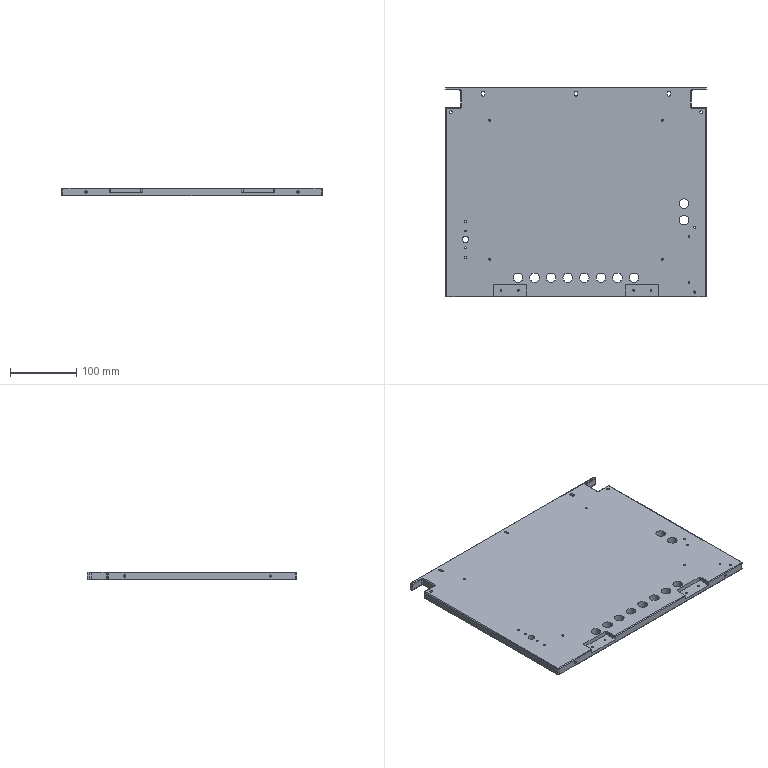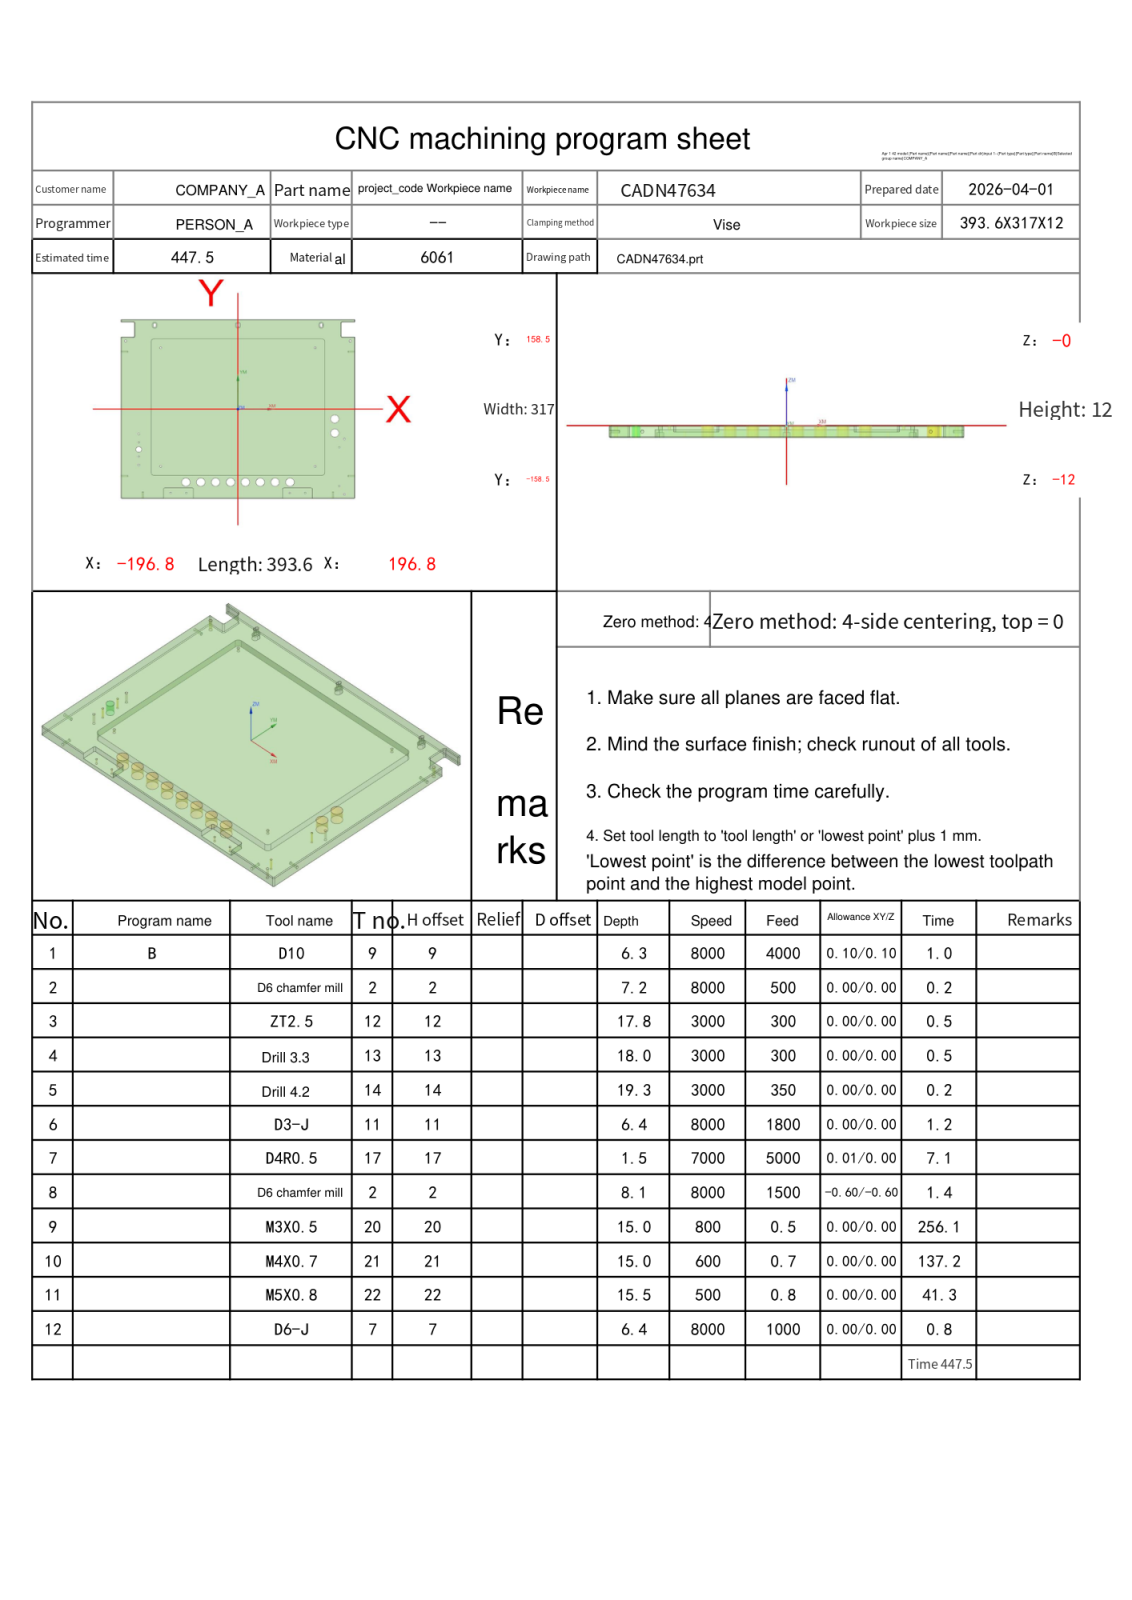NC program | NX | posted by the shop | part box 393.6 x 317 x 12 mm
Lines 5063 to 6733 of 6733:
N7 T17 M06
(D4R0.5  D=4. R=0.5 H=17 ce=0.01 di=0.00)
G00 G90 G54 X-120.803 Y-159.316 M03 S7000
G43 H17 Z10.01
M08
Z.488
G01 Z-.012 F5000.
X-123.9 Y-159.089
G03 X-124.138 Y-159.081 I-.238 J-3.254
X-125. Y-159.197 I0.0 J-3.263
G01 X-194.8
G02 X-197.497 Y-156.5 I0.0 J2.697
G01 Y126.5
G02 X-195.8 Y128.196 I1.697 J0.0
G01 X-175.9
G03 X-174.597 Y129.5 I0.0 J1.303
G01 Y152.
G03 X-175.9 Y153.304 I-1.303 J0.0
G01 X-195.8
G02 X-197.497 Y155.001 I0.0 J1.697
G01 Y157.5
G02 X-195.8 Y159.197 I1.697 J0.0
G01 X195.8
G02 X197.497 Y157.5 I0.0 J-1.697
G01 Y155.001
G02 X195.8 Y153.304 I-1.697 J0.0
G01 X175.9
G03 X174.597 Y152. I0.0 J-1.303
G01 Y129.5
G03 X175.9 Y128.196 I1.303 J0.0
G01 X195.8
G02 X197.497 Y126.5 I0.0 J-1.697
G01 Y-156.5
G02 X194.8 Y-159.197 I-2.697 J0.0
G01 X125.
X124.799 Y-159.126
X123.899 Y-159.084
Y-159.152 Z-.018
X123.9 Z-.025
X125. Y-159.284
X194.8
G03 X197.584 Y-156.5 I0.0 J2.784
G01 Y126.5
G03 X195.8 Y128.284 I-1.784 J0.0
G01 X175.9
G02 X174.685 Y129.5 I0.0 J1.216
G01 Y152.
G02 X175.9 Y153.216 I1.216 J0.0
G01 X195.8
G03 X197.584 Y155.001 I0.0 J1.784
G01 Y157.5
G03 X195.8 Y159.284 I-1.784 J0.0
G01 X-195.8
G03 X-197.584 Y157.5 I0.0 J-1.784
G01 Y155.001
G03 X-195.8 Y153.216 I1.784 J0.0
G01 X-175.9
G02 X-174.685 Y152. I0.0 J-1.216
G01 Y129.5
G02 X-175.9 Y128.284 I-1.216 J0.0
G01 X-195.8
G03 X-197.584 Y126.5 I0.0 J-1.784
G01 Y-156.5
G03 X-194.8 Y-159.284 I2.784 J0.0
G01 X-125.
G02 X-124.067 Y-159.161 I.932 J-3.463
G01 X-123.9 Y-159.165
Y-159.243 Z-.034
Y-159.259 Z-.042
X-124.07 Y-159.255
G03 X-125. Y-159.363 I0.0 J-4.044
G01 X-194.8
G02 X-197.663 Y-156.5 I0.0 J2.863
G01 Y126.5
G02 X-195.8 Y128.363 I1.863 J0.0
G01 X-175.9
G03 X-174.764 Y129.5 I0.0 J1.137
G01 Y152.
G03 X-175.9 Y153.137 I-1.137 J0.0
G01 X-195.8
G02 X-197.663 Y155.001 I0.0 J1.863
G01 Y157.5
G02 X-195.8 Y159.363 I1.863 J0.0
G01 X195.8
G02 X197.663 Y157.5 I0.0 J-1.863
G01 Y155.001
G02 X195.8 Y153.137 I-1.863 J0.0
G01 X175.9
G03 X174.764 Y152. I0.0 J-1.137
G01 Y129.5
G03 X175.9 Y128.363 I1.137 J0.0
G01 X195.8
G02 X197.663 Y126.5 I0.0 J-1.863
G01 Y-156.5
G02 X194.8 Y-159.363 I-2.863 J0.0
G01 X125.
X123.9 Y-159.238
Y-159.293 Z-.053
Y-159.329 Z-.063
X123.949 Y-159.333
X125. Y-159.44
X194.8
G03 X197.74 Y-156.5 I0.0 J2.94
G01 Y126.5
G03 X195.8 Y128.44 I-1.94 J0.0
G01 X175.9
G02 X174.84 Y129.5 I0.0 J1.06
G01 Y152.
G02 X175.9 Y153.06 I1.06 J0.0
G01 X195.8 Y153.061
G03 X197.74 Y155.001 I0.0 J1.94
G01 Y157.5
G03 X195.8 Y159.44 I-1.94 J0.0
G01 X-195.8
G03 X-197.74 Y157.5 I0.0 J-1.94
G01 Y155.001
G03 X-195.8 Y153.061 I1.94 J0.0
G01 X-175.9 Y153.06
G02 X-174.84 Y152. I0.0 J-1.06
G01 Y129.5
G02 X-175.9 Y128.44 I-1.06 J0.0
G01 X-195.8
G03 X-197.74 Y126.5 I0.0 J-1.94
G01 Y-156.5
G03 X-194.8 Y-159.44 I2.94 J0.0
G01 X-125.
G02 X-124.019 Y-159.344 I.981 J-4.998
G01 X-123.9 Y-159.346
X-123.899 Y-159.394 Z-.076
Y-159.426 Z-.089
G03 X-124.115 Y-159.42 I-.216 J-4.053
X-125. Y-159.518 I0.0 J-4.059
G01 X-194.8
G02 X-197.818 Y-156.5 I0.0 J3.018
G01 Y126.5
G02 X-195.8 Y128.518 I2.018 J0.0
G01 X-175.9
G03 X-174.918 Y129.5 I0.0 J.982
G01 Y152.
G03 X-175.9 Y152.982 I-.982 J0.0
G01 X-195.8 Y152.983
G02 X-197.818 Y155.001 I0.0 J2.018
G01 Y157.5
G02 X-195.8 Y159.518 I2.018 J0.0
G01 X195.8
G02 X197.818 Y157.5 I0.0 J-2.018
G01 Y155.001
G02 X195.8 Y152.983 I-2.018 J0.0
G01 X175.9 Y152.982
G03 X174.918 Y152. I0.0 J-.982
G01 Y129.5
G03 X175.9 Y128.518 I.982 J0.0
G01 X195.8
G02 X197.818 Y126.5 I0.0 J-2.018
G01 Y-156.5
G02 X194.8 Y-159.518 I-3.018 J0.0
G01 X125.
G03 X123.898 Y-159.403 I-1.187 J-6.06
G01 Y-159.446 Z-.104
Y-159.483 Z-.12
G02 X125. Y-159.597 I-.142 J-6.724
G01 X194.8
G03 X197.897 Y-156.5 I0.0 J3.097
G01 Y126.5
G03 X195.8 Y128.597 I-2.097 J0.0
G01 X175.9
G02 X174.997 Y129.5 I0.0 J.903
G01 Y152.
G02 X175.9 Y152.903 I.903 J0.0
G01 X195.8 Y152.904
G03 X197.897 Y155.001 I0.0 J2.097
G01 Y157.5
G03 X195.8 Y159.597 I-2.097 J0.0
G01 X-195.8
G03 X-197.897 Y157.5 I0.0 J-2.097
G01 Y155.001
G03 X-195.8 Y152.904 I2.097 J0.0
G01 X-175.9 Y152.903
G02 X-174.997 Y152. I0.0 J-.903
G01 Y129.5
G02 X-175.9 Y128.597 I-.903 J0.0
G01 X-195.8
G03 X-197.897 Y126.5 I0.0 J-2.097
G01 Y-156.5
G03 X-194.8 Y-159.597 I3.097 J0.0
G01 X-125.
G02 X-124.051 Y-159.497 I.949 J-4.449
G01 X-123.899 Y-159.5
X-123.9 Y-159.542 Z-.138
Y-159.576 Z-.156
G03 X-125. Y-159.677 I.01 J-6.176
G01 X-194.8
G02 X-197.977 Y-156.5 I0.0 J3.177
G01 Y126.5
G02 X-195.8 Y128.676 I2.177 J0.0
G01 X-175.9
G03 X-175.077 Y129.5 I0.0 J.823
G01 Y152.
G03 X-175.9 Y152.824 I-.823 J0.0
G01 X-195.8
G02 X-197.977 Y155.001 I0.0 J2.177
G01 Y157.5
G02 X-195.8 Y159.677 I2.177 J0.0
G01 X195.8
G02 X197.977 Y157.5 I0.0 J-2.177
G01 Y155.001
G02 X195.8 Y152.824 I-2.177 J0.0
G01 X175.9
G03 X175.077 Y152. I0.0 J-.823
G01 Y129.5
G03 X175.9 Y128.676 I.823 J0.0
G01 X195.8
G02 X197.977 Y126.5 I0.0 J-2.177
G01 Y-156.5
G02 X194.8 Y-159.677 I-3.177 J0.0
G01 X125.
G03 X123.9 Y-159.565 I-1.385 J-8.202
G01 X123.899 Y-159.615 Z-.177
Y-159.657 Z-.198
G02 X125. Y-159.755 I-.262 J-9.172
G01 X194.8
G03 X198.055 Y-156.5 I0.0 J3.255
G01 Y126.5
G03 X195.8 Y128.755 I-2.255 J0.0
G01 X175.9
G02 X175.155 Y129.5 I0.0 J.745
G01 Y152.
G02 X175.9 Y152.745 I.745 J0.0
G01 X195.8 Y152.746
G03 X198.055 Y155.001 I0.0 J2.255
G01 Y157.5
G03 X195.8 Y159.755 I-2.255 J0.0
G01 X-195.8
G03 X-198.055 Y157.5 I0.0 J-2.255
G01 Y155.001
G03 X-195.8 Y152.746 I2.255 J0.0
G01 X-175.9 Y152.745
G02 X-175.155 Y152. I0.0 J-.745
G01 Y129.5
G02 X-175.9 Y128.755 I-.745 J0.0
G01 X-195.8
G03 X-198.055 Y126.5 I0.0 J-2.255
G01 Y-156.5
G03 X-194.8 Y-159.755 I3.255 J0.0
G01 X-125.
G02 X-123.899 Y-159.661 I1.326 J-9.063
G01 Y-159.71 Z-.222
Y-159.753 Z-.247
G03 X-125. Y-159.834 I.089 J-8.636
G01 X-194.8
G02 X-198.134 Y-156.5 I0.0 J3.334
G01 Y126.5
G02 X-195.8 Y128.834 I2.334 J0.0
G01 X-175.9
G03 X-175.235 Y129.5 I0.0 J.666
G01 Y152.
G03 X-175.9 Y152.666 I-.666 J0.0
G01 X-195.8
G02 X-198.134 Y155.001 I0.0 J2.334
G01 Y157.5
G02 X-195.8 Y159.834 I2.334 J0.0
G01 X195.8
G02 X198.134 Y157.5 I0.0 J-2.334
G01 Y155.001
G02 X195.8 Y152.666 I-2.334 J0.0
G01 X175.9
G03 X175.235 Y152. I0.0 J-.666
G01 Y129.5
G03 X175.9 Y128.834 I.666 J0.0
G01 X195.8
G02 X198.134 Y126.5 I0.0 J-2.334
G01 Y-156.5
G02 X194.8 Y-159.834 I-3.334 J0.0
G01 X125.
G03 X123.899 Y-159.752 I-1.11 J-7.483
G01 Y-159.794 Z-.274
X123.9 Y-159.827 Z-.301
G02 X125. Y-159.912 I-.128 J-8.894
G01 X194.8
G03 X198.212 Y-156.5 I0.0 J3.412
G01 Y126.5
G03 X195.8 Y128.912 I-2.412 J0.0
G01 X175.9
G02 X175.312 Y129.5 I0.0 J.588
G01 Y152.
G02 X175.9 Y152.588 I.588 J0.0
G01 X195.8 Y152.589
G03 X198.212 Y155.001 I0.0 J2.412
G01 Y157.5
G03 X195.8 Y159.912 I-2.412 J0.0
G01 X-195.8
G03 X-198.212 Y157.5 I0.0 J-2.412
G01 Y155.001
G03 X-195.8 Y152.589 I2.412 J0.0
G01 X-175.9 Y152.588
G02 X-175.312 Y152. I0.0 J-.588
G01 Y129.5
G02 X-175.9 Y128.912 I-.588 J0.0
G01 X-195.8
G03 X-198.212 Y126.5 I0.0 J-2.412
G01 Y-156.5
G03 X-194.8 Y-159.912 I3.412 J0.0
G01 X-125.
G02 X-123.9 Y-159.827 I1.229 J-8.808
G01 Y-159.872 Z-.331
Y-159.908 Z-.361
G03 X-125. Y-159.986 I.01 J-7.869
G01 X-194.8
G02 X-198.286 Y-156.5 I0.0 J3.486
G01 Y126.5
G02 X-195.8 Y128.986 I2.486 J0.0
G01 X-175.9
G03 X-175.386 Y129.5 I0.0 J.514
G01 Y152.
G03 X-175.9 Y152.514 I-.514 J0.0
G01 X-195.8 Y152.515
G02 X-198.286 Y155.001 I0.0 J2.486
G01 Y157.5
G02 X-195.8 Y159.986 I2.486 J0.0
G01 X195.8
G02 X198.286 Y157.5 I0.0 J-2.486
G01 Y155.001
G02 X195.8 Y152.515 I-2.486 J0.0
G01 X175.9 Y152.514
G03 X175.386 Y152. I0.0 J-.514
G01 Y129.5
G03 X175.9 Y128.986 I.514 J0.0
G01 X195.8
G02 X198.286 Y126.5 I0.0 J-2.486
G01 Y-156.5
G02 X194.8 Y-159.986 I-3.486 J0.0
G01 X125.
G03 X123.9 Y-159.908 I-1.11 J-7.791
G01 X123.899 Y-159.953 Z-.394
Y-159.991 Z-.426
G02 X125. Y-160.058 I-.091 J-10.664
G01 X194.8
G03 X198.358 Y-156.5 I0.0 J3.558
G01 Y126.5
G03 X195.8 Y129.057 I-2.558 J0.0
G01 X175.9
G02 X175.458 Y129.5 I0.0 J.442
G01 Y152.
G02 X175.9 Y152.443 I.442 J0.0
G01 X195.8
G03 X198.358 Y155.001 I0.0 J2.558
G01 Y157.5
G03 X195.8 Y160.058 I-2.558 J0.0
G01 X-195.8
G03 X-198.358 Y157.5 I0.0 J-2.558
G01 Y155.001
G03 X-195.8 Y152.443 I2.558 J0.0
G01 X-175.9
G02 X-175.458 Y152. I0.0 J-.442
G01 Y129.5
G02 X-175.9 Y129.057 I-.442 J0.0
G01 X-195.8
G03 X-198.358 Y126.5 I0.0 J-2.558
G01 Y-156.5
G03 X-194.8 Y-160.058 I3.558 J0.0
G01 X-125.
G02 X-123.899 Y-159.991 I1.192 J-10.596
G01 Y-160.03 Z-.462
Y-160.06 Z-.497
X-123.956
G03 X-125. Y-160.125 I0.0 J-8.34
G01 X-194.8
G02 X-198.425 Y-156.5 I0.0 J3.625
G01 Y126.5
G02 X-195.8 Y129.125 I2.625 J0.0
G01 X-175.9
G03 X-175.525 Y129.5 I0.0 J.375
G01 Y152.
G03 X-175.9 Y152.375 I-.375 J0.0
G01 X-195.8
G02 X-198.425 Y155.001 I0.0 J2.625
G01 Y157.5
G02 X-195.8 Y160.125 I2.625 J0.0
G01 X195.8
G02 X198.425 Y157.5 I0.0 J-2.625
G01 Y155.001
G02 X195.8 Y152.375 I-2.625 J0.0
G01 X175.9
G03 X175.525 Y152. I0.0 J-.375
G01 Y129.5
G03 X175.9 Y129.125 I.375 J0.0
G01 X195.8
G02 X198.425 Y126.5 I0.0 J-2.625
G01 Y-156.5
G02 X194.8 Y-160.125 I-3.625 J0.0
G01 X125.
G03 X123.956 Y-160.06 I-1.044 J-8.275
G01 X123.899
X123.9 Y-160.097 Z-.535
Y-160.122 Z-.572
G02 X125. Y-160.189 I-.149 J-11.663
G01 X194.8
G03 X198.489 Y-156.5 I0.0 J3.689
G01 Y126.5
G03 X195.8 Y129.188 I-2.689 J0.0
G01 X175.9
G02 X175.589 Y129.5 I0.0 J.311
G01 Y152.
G02 X175.9 Y152.312 I.311 J0.0
G01 X195.8
G03 X198.489 Y155.001 I0.0 J2.689
G01 Y157.5
G03 X195.8 Y160.189 I-2.689 J0.0
G01 X-195.8
G03 X-198.489 Y157.5 I0.0 J-2.689
G01 Y155.001
G03 X-195.8 Y152.312 I2.689 J0.0
G01 X-175.9
G02 X-175.589 Y152. I0.0 J-.311
G01 Y129.5
G02 X-175.9 Y129.188 I-.311 J0.0
G01 X-195.8
G03 X-198.489 Y126.5 I0.0 J-2.689
G01 Y-156.5
G03 X-194.8 Y-160.189 I3.689 J0.0
G01 X-125.
G02 X-123.9 Y-160.122 I1.249 J-11.596
G01 Y-160.158 Z-.612
Y-160.186 Z-.651
X-124.003
G03 X-125. Y-160.247 I0.0 J-8.137
G01 X-194.8
G02 X-198.547 Y-156.5 I0.0 J3.747
G01 Y126.5
G02 X-195.8 Y129.247 I2.747 J0.0
G01 X-175.9
G03 X-175.647 Y129.5 I0.0 J.253
G01 Y152.
G03 X-175.9 Y152.253 I-.253 J0.0
G01 X-195.8 Y152.254
G02 X-198.547 Y155.001 I0.0 J2.747
G01 Y157.5
G02 X-195.8 Y160.247 I2.747 J0.0
G01 X195.8
G02 X198.547 Y157.5 I0.0 J-2.747
G01 Y155.001
G02 X195.8 Y152.254 I-2.747 J0.0
G01 X175.9 Y152.253
G03 X175.647 Y152. I0.0 J-.253
G01 Y129.5
G03 X175.9 Y129.247 I.253 J0.0
G01 X195.8
G02 X198.547 Y126.5 I0.0 J-2.747
G01 Y-156.5
G02 X194.8 Y-160.247 I-3.747 J0.0
G01 X125.
G03 X124.003 Y-160.186 I-.997 J-8.075
G01 X123.9
X123.899 Y-160.22 Z-.693
Y-160.246 Z-.735
X123.979
G02 X125. Y-160.3 I0.0 J-9.614
G01 X194.8
G03 X198.6 Y-156.5 I0.0 J3.8
G01 Y126.5
G03 X195.8 Y129.3 I-2.8 J0.0
G01 X175.9
G02 X175.7 Y129.5 I0.0 J.2
G01 Y152.
G02 X175.9 Y152.2 I.2 J0.0
G01 X195.8 Y152.201
G03 X198.6 Y155.001 I0.0 J2.8
G01 Y157.5
G03 X195.8 Y160.3 I-2.8 J0.0
G01 X-195.8
G03 X-198.6 Y157.5 I0.0 J-2.8
G01 Y155.001
G03 X-195.8 Y152.201 I2.8 J0.0
G01 X-175.9 Y152.2
G02 X-175.7 Y152. I0.0 J-.2
G01 Y129.5
G02 X-175.9 Y129.3 I-.2 J0.0
G01 X-195.8
G03 X-198.6 Y126.5 I0.0 J-2.8
G01 Y-156.5
G03 X-194.8 Y-160.3 I3.8 J0.0
G01 X-125.
G02 X-123.977 Y-160.246 I1.023 J-9.576
G01 X-123.899
Y-160.272 Z-.778
X-123.898 Y-160.296 Z-.822
G03 X-125. Y-160.348 I.004 J-11.898
G01 X-194.8
G02 X-198.648 Y-156.5 I0.0 J3.848
G01 Y126.5
G02 X-195.8 Y129.348 I2.848 J0.0
G01 X-175.9
G03 X-175.748 Y129.5 I0.0 J.152
G01 Y152.
G03 X-175.9 Y152.152 I-.152 J0.0
G01 X-195.8 Y152.153
G02 X-198.648 Y155.001 I0.0 J2.848
G01 Y157.5
G02 X-195.8 Y160.348 I2.848 J0.0
G01 X195.8
G02 X198.648 Y157.5 I0.0 J-2.848
G01 Y155.001
G02 X195.8 Y152.153 I-2.848 J0.0
G01 X175.9 Y152.152
G03 X175.748 Y152. I0.0 J-.152
G01 Y129.5
G03 X175.9 Y129.348 I.152 J0.0
G01 X195.8
G02 X198.648 Y126.5 I0.0 J-2.848
G01 Y-156.5
G02 X194.8 Y-160.348 I-3.848 J0.0
G01 X125.
G03 X123.926 Y-160.297 I-1.074 J-11.297
G01 X123.899
Y-160.323 Z-.867
Y-160.342 Z-.912
G02 X124.143 Y-160.338 I.244 J-8.366
X124.516 Y-160.347 I0.0 J-8.369
G03 X125. Y-160.39 I.616 J4.15
G01 X194.8
G03 X198.69 Y-156.5 I0.0 J3.89
G01 Y126.5
G03 X195.8 Y129.39 I-2.89 J0.0
G01 X175.9
X175.84 Y129.396
X175.796 Y129.44
X175.79 Y129.5
Y152.
X175.796 Y152.06
X175.84 Y152.104
X175.9 Y152.11
X195.8 Y152.111
G03 X198.69 Y155.001 I0.0 J2.89
G01 Y157.5
G03 X195.8 Y160.39 I-2.89 J0.0
G01 X-195.8
G03 X-198.69 Y157.5 I0.0 J-2.89
G01 Y155.001
G03 X-195.8 Y152.111 I2.89 J0.0
G01 X-175.9 Y152.11
X-175.84 Y152.104
X-175.796 Y152.06
X-175.79 Y152.
Y129.5
X-175.796 Y129.44
X-175.84 Y129.396
X-175.9 Y129.39
X-195.8
G03 X-198.69 Y126.5 I0.0 J-2.89
G01 Y-156.5
G03 X-194.8 Y-160.39 I3.89 J0.0
G01 X-125.
G03 X-124.516 Y-160.349 I-.173 J4.958
G01 X-123.899 Y-160.336
Y-160.36 Z-.959
Y-160.374 Z-1.005
X-123.91
G03 X-125. Y-160.426 I0.0 J-11.544
G01 X-194.8
G02 X-198.726 Y-156.5 I0.0 J3.926
G01 Y126.5
G02 X-195.8 Y129.426 I2.926 J0.0
G01 X-175.9
X-175.858 Y129.427
X-175.827 Y129.458
X-175.826 Y129.5
Y152.
X-175.827 Y152.042
X-175.858 Y152.073
X-175.9 Y152.074
X-195.8 Y152.075
G02 X-198.726 Y155.001 I0.0 J2.926
G01 Y157.5
G02 X-195.8 Y160.426 I2.926 J0.0
G01 X195.8
G02 X198.726 Y157.5 I0.0 J-2.926
G01 Y155.001
G02 X195.8 Y152.075 I-2.926 J0.0
G01 X175.9 Y152.074
X175.858 Y152.073
X175.827 Y152.042
X175.826 Y152.
Y129.5
X175.827 Y129.458
X175.858 Y129.427
X175.9 Y129.426
X195.8
G02 X198.726 Y126.5 I0.0 J-2.926
G01 Y-156.5
G02 X194.8 Y-160.426 I-3.926 J0.0
G01 X125.
X124.666 Y-160.397
G03 X124.199 Y-160.376 I-.466 J-5.296
X123.899 Y-160.385 I0.0 J-5.317
G01 X123.9 Y-160.412 Z-1.053
Y-160.422 Z-1.1
G02 X124.216 Y-160.417 I.317 J-9.912
X124.516 Y-160.421 I0.0 J-9.917
G03 X125. Y-160.456 I.618 J5.232
G01 X194.8
G03 X198.756 Y-156.5 I0.0 J3.956
G01 Y126.5
G03 X195.8 Y129.456 I-2.956 J0.0
G01 X175.9
X175.873 Y129.453
X175.853 Y129.473
X175.856 Y129.5
Y152.
X175.853 Y152.027
X175.873 Y152.047
X175.9 Y152.044
X195.8 Y152.045
G03 X198.756 Y155.001 I0.0 J2.956
G01 Y157.5
G03 X195.8 Y160.456 I-2.956 J0.0
G01 X-195.8
G03 X-198.756 Y157.5 I0.0 J-2.956
G01 Y155.001
G03 X-195.8 Y152.045 I2.956 J0.0
G01 X-175.9 Y152.044
X-175.873 Y152.047
X-175.853 Y152.027
X-175.856 Y152.
Y129.5
X-175.853 Y129.473
X-175.873 Y129.453
X-175.9 Y129.456
X-195.8
G03 X-198.756 Y126.5 I0.0 J-2.956
G01 Y-156.5
G03 X-194.8 Y-160.456 I3.956 J0.0
G01 X-125.
G02 X-123.9 Y-160.413 I1.382 J-21.397
G01 Y-160.436 Z-1.149
Y-160.45 Z-1.198
X-124.799 Y-160.471
X-125. Y-160.479
X-194.8
G02 X-198.779 Y-156.5 I0.0 J3.979
G01 Y126.5
G02 X-195.8 Y129.479 I2.979 J0.0
G01 X-175.9
X-175.878 Y129.478
X-175.879 Y129.5
Y152.
X-175.878 Y152.022
X-175.9 Y152.021
X-195.8 Y152.022
G02 X-198.779 Y155.001 I0.0 J2.979
G01 Y157.5
G02 X-195.8 Y160.479 I2.979 J0.0
G01 X195.8
G02 X198.779 Y157.5 I0.0 J-2.979
G01 Y155.001
G02 X195.8 Y152.022 I-2.979 J0.0
G01 X175.9 Y152.021
X175.878 Y152.022
X175.879 Y152.
Y129.5
X175.878 Y129.478
X175.9 Y129.479
X195.8
G02 X198.779 Y126.5 I0.0 J-2.979
G01 Y-156.5
G02 X194.8 Y-160.479 I-3.979 J0.0
G01 X125.
G03 X124.184 Y-160.452 I-.816 J-12.346
X123.901 Y-160.455 I0.0 J-12.373
G01 X123.902 Y-160.469 Z-1.235
Y-160.475 Z-1.273
G02 X124.157 Y-160.473 I.255 J-18.193
X125. Y-160.493 I0.0 J-18.194
G01 X194.8
G03 X198.793 Y-156.5 I0.0 J3.993
G01 Y126.5
G03 X195.8 Y129.493 I-2.993 J0.0
G01 X175.9
X175.892 Y129.492
X175.893 Y129.5
Y152.
X175.892 Y152.008
X175.9 Y152.007
X195.8 Y152.008
G03 X198.793 Y155.001 I0.0 J2.993
G01 Y157.5
G03 X195.8 Y160.493 I-2.993 J0.0
G01 X-195.8
G03 X-198.793 Y157.5 I0.0 J-2.993
G01 Y155.001
G03 X-195.8 Y152.008 I2.993 J0.0
G01 X-175.9 Y152.007
X-175.892 Y152.008
X-175.893 Y152.
Y129.5
X-175.892 Y129.492
X-175.9 Y129.493
X-195.8
G03 X-198.793 Y126.5 I0.0 J-2.993
G01 Y-156.5
G03 X-194.8 Y-160.493 I3.993 J0.0
G01 X-125.
X-124.799 Y-160.484
X-123.902 Y-160.47
X-123.903 Y-160.481 Z-1.311
X-123.904 Y-160.485 Z-1.349
X-123.949 Y-160.488
X-124.799 Y-160.493
X-125. Y-160.502
X-194.8
G02 X-198.802 Y-156.5 I0.0 J4.002
G01 Y126.5
G02 X-195.8 Y129.502 I3.002 J0.0
G01 X-175.902
Y151.998
X-195.8
G02 X-198.802 Y155.001 I0.0 J3.002
G01 Y157.5
G02 X-195.8 Y160.502 I3.002 J0.0
G01 X195.8
G02 X198.802 Y157.5 I0.0 J-3.002
G01 Y155.001
G02 X195.8 Y151.998 I-3.002 J0.0
G01 X175.902
Y129.502
X195.8
G02 X198.802 Y126.5 I0.0 J-3.002
G01 Y-156.5
G02 X194.8 Y-160.502 I-4.002 J0.0
G01 X125.
X124.799 Y-160.493
X123.905 Y-160.487
X123.906 Y-160.495 Z-1.387
X123.907 Y-160.5 Z-1.424
X123.949 Y-160.502
X124.799 Y-160.503
X125. Y-160.508
X194.8
G03 X198.808 Y-156.5 I0.0 J4.008
G01 Y126.5
G03 X195.8 Y129.508 I-3.008 J0.0
G01 X175.908
Y151.992
X195.8 Y151.993
G03 X198.808 Y155.001 I0.0 J3.008
G01 Y157.5
G03 X195.8 Y160.508 I-3.008 J0.0
G01 X-195.8
G03 X-198.808 Y157.5 I0.0 J-3.008
G01 Y155.001
G03 X-195.8 Y151.993 I3.008 J0.0
G01 X-175.908 Y151.992
Y129.508
X-195.8
G03 X-198.808 Y126.5 I0.0 J-3.008
G01 Y-156.5
G03 X-194.8 Y-160.508 I4.008 J0.0
G01 X-125.
X-124.799 Y-160.503
X-123.949 Y-160.501
X-123.906 Y-160.499
X-123.909 Y-160.507 Z-1.5
X-194.81 Y-160.51
G02 X-198.744 Y-157.224 I.011 J4.011
X-198.81 Y-156.5 I3.97 J.724
G01 X-198.807 Y126.638
G02 X-196.194 Y129.484 I3.007 J-.139
X-195.818 Y129.509 I.376 J-2.828
G01 X-195.81
X-175.924 Y129.51
X-175.912 Y129.513
X-175.911 Y129.525
Y151.988
X-175.925 Y151.99
X-177.495
X-195.8 Y151.991
G02 X-198.796 Y154.708 I0.0 J3.01
G01 X-198.806 Y154.862
X-198.809 Y154.991
X-198.81 Y157.5
X-198.806 Y157.646
G02 X-195.969 Y160.505 I3.006 J-.146
G01 X195.8 Y160.51
X196.045 Y160.5
G02 X198.806 Y157.646 I-.245 J-3.
G01 X198.81 Y157.5
X198.809 Y154.991
X198.807 Y154.862
G02 X195.944 Y151.994 I-3.007 J.138
G01 X175.911 Y151.988
X175.91 Y151.958
X175.911 Y129.525
X175.912 Y129.513
X175.924 Y129.51
X195.81 Y129.509
X195.813
G02 X196.194 Y129.484 I0.0 J-2.922
X198.807 Y126.638 I-.394 J-2.984
G01 X198.81 Y-156.505
G02 X198.742 Y-157.234 I-3.98 J0.0
X194.81 Y-160.51 I-3.943 J.735
G01 X123.91 Y-160.507
G00 Z10.01
X79.118 Y-159.445
Z.488
G01 Z-.012
X76.1 Y-159.087
X75. Y-159.197
X-75.
G03 X-75.963 Y-159.08 I-.963 J-3.914
G01 X-76.1 Y-159.082
Y-159.149 Z-.025
X-75. Y-159.284
X75.
X76.1 Y-159.159
Y-159.235 Z-.034
Y-159.249 Z-.042
X75. Y-159.363
X-75.
X-76.1 Y-159.231
Y-159.285 Z-.053
Y-159.322 Z-.063
X-75. Y-159.44
X75.
G02 X76.1 Y-159.339 I1.134 J-6.292
G01 X76.101 Y-159.384 Z-.076
Y-159.417 Z-.089
X76.006 Y-159.416
G03 X75. Y-159.518 I0.0 J-5.045
G01 X-75.
X-76.069 Y-159.389
X-76.1 Y-159.387
Y-159.437 Z-.104
Y-159.466 Z-.12
X-75. Y-159.597
X75.
G02 X76.026 Y-159.494 I1.026 J-5.055
G01 X76.101 Y-159.495
X76.1 Y-159.537 Z-.138
Y-159.573 Z-.156
G03 X75. Y-159.677 I.042 J-6.341
G01 X-75.
G03 X-76.1 Y-159.559 I-1.59 J-9.655
G01 Y-159.613 Z-.177
X-76.101 Y-159.656 Z-.198
G02 X-75. Y-159.755 I-.281 J-9.276
G01 X75.
G02 X76.101 Y-159.661 I1.247 J-8.074
G01 Y-159.709 Z-.222
Y-159.753 Z-.247
G03 X75. Y-159.834 I.005 J-7.561
G01 X-75.
G03 X-76.101 Y-159.753 I-1.106 J-7.483
G01 Y-159.794 Z-.274
Y-159.828 Z-.301
G02 X-75. Y-159.912 I-.126 J-8.941
G01 X75.
G02 X76.1 Y-159.828 I1.227 J-8.856
G01 Y-159.872 Z-.331
Y-159.908 Z-.361
G03 X75. Y-159.986 I0.0 J-7.79
G01 X-75.
G03 X-76.099 Y-159.908 I-1.099 J-7.713
G01 X-76.101 Y-159.953 Z-.394
X-76.102 Y-159.992 Z-.426
G02 X-75. Y-160.058 I-.06 J-10.274
G01 X75.
G02 X76.101 Y-159.992 I1.161 J-10.207
G01 Y-160.03 Z-.462
Y-160.06 Z-.497
X76.034
G03 X75. Y-160.125 I0.0 J-8.236
G01 X-75.
G03 X-76.034 Y-160.06 I-1.034 J-8.172
G01 X-76.101
Y-160.097 Z-.535
X-76.1 Y-160.123 Z-.572
G02 X-75. Y-160.189 I-.123 J-11.351
G01 X75.
G02 X76.1 Y-160.123 I1.223 J-11.284
G01 Y-160.158 Z-.612
Y-160.187 Z-.651
X75.983 Y-160.186
G03 X75. Y-160.247 I0.0 J-7.968
G01 X-75.
G03 X-75.982 Y-160.186 I-.982 J-7.905
G01 X-76.1 Y-160.187
X-76.101 Y-160.22 Z-.693
Y-160.247 Z-.735
X-75.997 Y-160.246
G02 X-75. Y-160.3 I0.0 J-9.222
G01 X75.
G02 X75.999 Y-160.246 I.999 J-9.191
G01 X76.101 Y-160.247
X76.102 Y-160.272 Z-.778
Y-160.297 Z-.822
X76.074
G03 X75. Y-160.348 I0.0 J-11.388
G01 X-75.
G03 X-76.054 Y-160.298 I-1.054 J-11.047
G01 X-76.102
X-76.101 Y-160.322 Z-.867
Y-160.338 Z-.912
X-75.503 Y-160.346
G03 X-75. Y-160.39 I.682 J4.912
G01 X75.
G03 X75.503 Y-160.348 I-.22 J5.664
G01 X76.101 Y-160.335
Y-160.359 Z-.959
Y-160.373 Z-1.005
G03 X75. Y-160.426 I.018 J-11.906
G01 X-75.
X-75.503 Y-160.384
X-76.1 Y-160.378
Y-160.404 Z-1.053
Y-160.418 Z-1.1
X-75.503 Y-160.422
G03 X-75. Y-160.456 I.638 J5.776
G01 X75.
G02 X76.1 Y-160.412 I1.457 J-22.555
G01 Y-160.434 Z-1.149
Y-160.449 Z-1.198
X75.22 Y-160.471
X75. Y-160.479
X-75.
G03 X-75.916 Y-160.453 I-.916 J-15.962
G01 X-76.1 Y-160.454
X-76.099 Y-160.461 Z-1.235
Y-160.475 Z-1.273
X-75.22 Y-160.482
X-75. Y-160.493
X75.
X75.22 Y-160.484
X76.099 Y-160.469
Y-160.48 Z-1.311
X76.098 Y-160.485 Z-1.349
X75.22 Y-160.493
X75. Y-160.502
X-75.
X-75.22 Y-160.493
X-76.098 Y-160.487
Y-160.496 Z-1.387
X-76.097 Y-160.5 Z-1.424
X-75. Y-160.508
X75.
X76.097 Y-160.499
X76.096 Y-160.508 Z-1.5
X-76.095
G00 Z10.01
G91 G28 Z0.0
M05
M09
G91 G28 Z0.0
M01
N8 T02 M06
(D6 chamfer mill D=6. R=0. H=02 ce=-0.30 di=0.00)
G00 G90 G54 X-164.146 Y-68.114 M03 S7000
G43 H02 Z20.
M08
Z2.5
G01 X-164.155 Y-68.106 Z2.495 F1500.
X-164.511 Y-67.856 Z2.337
X-164.789 Y-67.696 Z2.22
X-165.183 Y-67.512 Z2.062
X-165.593 Y-67.37 Z1.904
X-166.016 Y-67.269 Z1.746
X-166.446 Y-67.212 Z1.588
X-166.88 Y-67.198 Z1.43
X-167.314 Y-67.228 Z1.272
X-167.742 Y-67.301 Z1.114
X-168.16 Y-67.418 Z.956
X-168.565 Y-67.576 Z.797
X-168.952 Y-67.773 Z.639
X-169.316 Y-68.009 Z.481
X-169.655 Y-68.281 Z.323
X-169.965 Y-68.585 Z.165
X-170.243 Y-68.919 Z.007
X-170.486 Y-69.279 Z-.151
X-170.691 Y-69.662 Z-.309
X-170.856 Y-70.064 Z-.467
X-170.98 Y-70.48 Z-.625
X-171.062 Y-70.907 Z-.783
X-171.1 Y-71.339 Z-.942
Y-71.5 Z-1.
G03 X-166.8 Y-75.8 I4.3 J0.0
X-162.5 Y-71.5 I0.0 J4.3
X-166.8 Y-67.2 I-4.3 J0.0
X-171.1 Y-71.5 I0.0 J-4.3
X-171.071 Y-71.999 I4.3 J0.0
G01 Z1.5
G00 Z20.
X-88.173 Y-122.982
Z2.5
G01 X-88.703 Y-123.058 Z2.305
X-89.244 Y-123.183 Z2.103
X-89.772 Y-123.354 Z1.901
X-90.284 Y-123.568 Z1.699
X-90.777 Y-123.825 Z1.497
X-91.245 Y-124.123 Z1.295
X-91.687 Y-124.459 Z1.093
X-92.098 Y-124.831 Z.891
X-92.477 Y-125.237 Z.689
X-92.82 Y-125.674 Z.487
X-93.125 Y-126.138 Z.285
X-93.389 Y-126.626 Z.082
X-93.611 Y-127.135 Z-.12
X-93.79 Y-127.661 Z-.322
X-93.923 Y-128.2 Z-.524
X-94.01 Y-128.748 Z-.726
X-94.05 Y-129.302 Z-.928
Y-129.5 Z-1.
G03 X-87.5 Y-136.05 I6.55 J0.0
X-80.95 Y-129.5 I0.0 J6.55
X-87.5 Y-122.95 I-6.55 J0.0
X-94.05 Y-129.5 I0.0 J-6.55
X-94.031 Y-130. I6.55 J0.0
G01 Z1.5
G00 Z20.
X-63.173 Y-122.982
Z2.5
G01 X-63.703 Y-123.058 Z2.305
X-64.244 Y-123.183 Z2.103
X-64.772 Y-123.354 Z1.901
X-65.284 Y-123.568 Z1.699
X-65.777 Y-123.825 Z1.497
X-66.245 Y-124.123 Z1.295
X-66.687 Y-124.459 Z1.093
X-67.098 Y-124.831 Z.891
X-67.477 Y-125.237 Z.689
X-67.82 Y-125.674 Z.487
X-68.125 Y-126.138 Z.285
X-68.389 Y-126.626 Z.082
X-68.611 Y-127.135 Z-.12
X-68.79 Y-127.661 Z-.322
X-68.923 Y-128.2 Z-.524
X-69.01 Y-128.748 Z-.726
X-69.05 Y-129.302 Z-.928
Y-129.5 Z-1.
G03 X-62.5 Y-136.05 I6.55 J0.0
X-55.95 Y-129.5 I0.0 J6.55
X-62.5 Y-122.95 I-6.55 J0.0
X-69.05 Y-129.5 I0.0 J-6.55
X-69.031 Y-130. I6.55 J0.0
G01 Z1.5
G00 Z20.
X-38.173 Y-122.982
Z2.5
G01 X-38.703 Y-123.058 Z2.305
X-39.244 Y-123.183 Z2.103
X-39.772 Y-123.354 Z1.901
X-40.284 Y-123.568 Z1.699
X-40.777 Y-123.825 Z1.497
X-41.245 Y-124.123 Z1.295
X-41.687 Y-124.459 Z1.093
X-42.098 Y-124.831 Z.891
X-42.477 Y-125.237 Z.689
X-42.82 Y-125.674 Z.487
X-43.125 Y-126.138 Z.285
X-43.389 Y-126.626 Z.082
X-43.611 Y-127.135 Z-.12
X-43.79 Y-127.661 Z-.322
X-43.923 Y-128.2 Z-.524
X-44.01 Y-128.748 Z-.726
X-44.05 Y-129.302 Z-.928
Y-129.5 Z-1.
G03 X-37.5 Y-136.05 I6.55 J0.0
X-30.95 Y-129.5 I0.0 J6.55
X-37.5 Y-122.95 I-6.55 J0.0
X-44.05 Y-129.5 I0.0 J-6.55
X-44.031 Y-130. I6.55 J0.0
G01 Z1.5
G00 Z20.
X-13.173 Y-122.982
Z2.5
G01 X-13.703 Y-123.058 Z2.305
X-14.244 Y-123.183 Z2.103
X-14.772 Y-123.354 Z1.901
X-15.284 Y-123.568 Z1.699
X-15.777 Y-123.825 Z1.497
X-16.245 Y-124.123 Z1.295
X-16.687 Y-124.459 Z1.093
X-17.098 Y-124.831 Z.891
X-17.477 Y-125.237 Z.689
X-17.82 Y-125.674 Z.487
X-18.125 Y-126.138 Z.285
X-18.389 Y-126.626 Z.082
X-18.611 Y-127.135 Z-.12
X-18.79 Y-127.661 Z-.322
X-18.923 Y-128.2 Z-.524
X-19.01 Y-128.748 Z-.726
X-19.05 Y-129.302 Z-.928
Y-129.5 Z-1.
G03 X-12.5 Y-136.05 I6.55 J0.0
X-5.95 Y-129.5 I0.0 J6.55
X-12.5 Y-122.95 I-6.55 J0.0
X-19.05 Y-129.5 I0.0 J-6.55
X-19.031 Y-130. I6.55 J0.0
G01 Z1.5
G00 Z20.
X11.827 Y-122.982
Z2.5
G01 X11.297 Y-123.058 Z2.305
X10.756 Y-123.183 Z2.103
X10.228 Y-123.354 Z1.901
X9.716 Y-123.568 Z1.699
X9.224 Y-123.825 Z1.497
X8.755 Y-124.123 Z1.295
X8.313 Y-124.459 Z1.093
X7.902 Y-124.831 Z.891
X7.523 Y-125.237 Z.689
X7.18 Y-125.674 Z.487
X6.875 Y-126.138 Z.285
X6.611 Y-126.626 Z.082
X6.389 Y-127.135 Z-.12
X6.21 Y-127.661 Z-.322
X6.077 Y-128.2 Z-.524
X5.99 Y-128.748 Z-.726
X5.95 Y-129.302 Z-.928
Y-129.5 Z-1.
G03 X12.5 Y-136.05 I6.55 J0.0
X19.05 Y-129.5 I0.0 J6.55
X12.5 Y-122.95 I-6.55 J0.0
X5.95 Y-129.5 I0.0 J-6.55
X5.969 Y-130. I6.55 J0.0
G01 Z1.5
G00 Z20.
X36.827 Y-122.982
Z2.5
G01 X36.297 Y-123.058 Z2.305
X35.756 Y-123.183 Z2.103
X35.228 Y-123.354 Z1.901
X34.716 Y-123.568 Z1.699
X34.224 Y-123.825 Z1.497
X33.755 Y-124.123 Z1.295
X33.313 Y-124.459 Z1.093
X32.902 Y-124.831 Z.891
X32.523 Y-125.237 Z.689
X32.18 Y-125.674 Z.487
X31.875 Y-126.138 Z.285
X31.611 Y-126.626 Z.082
X31.389 Y-127.135 Z-.12
X31.21 Y-127.661 Z-.322
X31.077 Y-128.2 Z-.524
X30.99 Y-128.748 Z-.726
X30.95 Y-129.302 Z-.928
Y-129.5 Z-1.
G03 X37.5 Y-136.05 I6.55 J0.0
X44.05 Y-129.5 I0.0 J6.55
X37.5 Y-122.95 I-6.55 J0.0
X30.95 Y-129.5 I0.0 J-6.55
X30.969 Y-130. I6.55 J0.0
G01 Z1.5
G00 Z20.
X61.827 Y-122.982
Z2.5
G01 X61.297 Y-123.058 Z2.305
X60.756 Y-123.183 Z2.103
X60.228 Y-123.354 Z1.901
X59.716 Y-123.568 Z1.699
X59.224 Y-123.825 Z1.497
X58.755 Y-124.123 Z1.295
X58.313 Y-124.459 Z1.093
X57.902 Y-124.831 Z.891
X57.523 Y-125.237 Z.689
X57.18 Y-125.674 Z.487
X56.875 Y-126.138 Z.285
X56.611 Y-126.626 Z.082
X56.389 Y-127.135 Z-.12
X56.21 Y-127.661 Z-.322
X56.077 Y-128.2 Z-.524
X55.99 Y-128.748 Z-.726
X55.95 Y-129.302 Z-.928
Y-129.5 Z-1.
G03 X62.5 Y-136.05 I6.55 J0.0
X69.05 Y-129.5 I0.0 J6.55
X62.5 Y-122.95 I-6.55 J0.0
X55.95 Y-129.5 I0.0 J-6.55
X55.969 Y-130. I6.55 J0.0
G01 Z1.5
G00 Z20.
X86.827 Y-122.982
Z2.5
G01 X86.297 Y-123.058 Z2.305
X85.756 Y-123.183 Z2.103
X85.228 Y-123.354 Z1.901
X84.716 Y-123.568 Z1.699
X84.224 Y-123.825 Z1.497
X83.755 Y-124.123 Z1.295
X83.313 Y-124.459 Z1.093
X82.902 Y-124.831 Z.891
X82.523 Y-125.237 Z.689
X82.18 Y-125.674 Z.487
X81.875 Y-126.138 Z.285
X81.611 Y-126.626 Z.082
X81.389 Y-127.135 Z-.12
X81.21 Y-127.661 Z-.322
X81.077 Y-128.2 Z-.524
X80.99 Y-128.748 Z-.726
X80.95 Y-129.302 Z-.928
Y-129.5 Z-1.
G03 X87.5 Y-136.05 I6.55 J0.0
X94.05 Y-129.5 I0.0 J6.55
X87.5 Y-122.95 I-6.55 J0.0
X80.95 Y-129.5 I0.0 J-6.55
X80.969 Y-130. I6.55 J0.0
G01 Z1.5
G00 Z20.
X162.127 Y-35.982
Z2.5
G01 X161.597 Y-36.058 Z2.305
X161.056 Y-36.183 Z2.103
X160.528 Y-36.354 Z1.901
X160.016 Y-36.568 Z1.699
X159.524 Y-36.825 Z1.497
X159.055 Y-37.123 Z1.295
X158.613 Y-37.459 Z1.093
X158.202 Y-37.831 Z.891
X157.823 Y-38.237 Z.689
X157.48 Y-38.674 Z.487
X157.175 Y-39.138 Z.285
X156.911 Y-39.626 Z.082
X156.689 Y-40.135 Z-.12
X156.51 Y-40.661 Z-.322
X156.377 Y-41.2 Z-.524
X156.29 Y-41.748 Z-.726
X156.25 Y-42.302 Z-.928
Y-42.5 Z-1.
G03 X162.8 Y-49.05 I6.55 J0.0
X169.35 Y-42.5 I0.0 J6.55
X162.8 Y-35.95 I-6.55 J0.0
X156.25 Y-42.5 I0.0 J-6.55
X156.269 Y-43. I6.55 J0.0
G01 Z1.5
G00 Z20.
X162.127 Y-10.982
Z2.5
G01 X161.597 Y-11.058 Z2.305
X161.056 Y-11.183 Z2.103
X160.528 Y-11.354 Z1.901
X160.016 Y-11.568 Z1.699
X159.524 Y-11.825 Z1.497
X159.055 Y-12.123 Z1.295
X158.613 Y-12.459 Z1.093
X158.202 Y-12.831 Z.891
X157.823 Y-13.237 Z.689
X157.48 Y-13.674 Z.487
X157.175 Y-14.138 Z.285
X156.911 Y-14.626 Z.082
X156.689 Y-15.135 Z-.12
X156.51 Y-15.661 Z-.322
X156.377 Y-16.2 Z-.524
X156.29 Y-16.748 Z-.726
X156.25 Y-17.302 Z-.928
Y-17.5 Z-1.
G03 X162.8 Y-24.05 I6.55 J0.0
X169.35 Y-17.5 I0.0 J6.55
X162.8 Y-10.95 I-6.55 J0.0
X156.25 Y-17.5 I0.0 J-6.55
X156.269 Y-18. I6.55 J0.0
G01 Z1.5
G00 Z20.
X141.55 Y148.258
Z2.5
G01 Y150.096 Z1.831
X141.515 Y150.343 Z1.74
X141.44 Y150.581 Z1.649
X141.329 Y150.804 Z1.558
X141.183 Y151.006 Z1.468
X141.006 Y151.183 Z1.377
X140.804 Y151.329 Z1.286
X140.581 Y151.44 Z1.195
X140.343 Y151.515 Z1.105
X140.096 Y151.55 Z1.014
X139.904 Z.944
X139.657 Y151.515 Z.853
X139.419 Y151.44 Z.762
X139.196 Y151.329 Z.672
X138.994 Y151.183 Z.581
X138.817 Y151.006 Z.49
X138.671 Y150.804 Z.399
X138.56 Y150.581 Z.309
X138.485 Y150.343 Z.218
X138.45 Y150.096 Z.127
Y147. Z-1.
G03 X140. Y145.45 I1.55 J0.0
X141.55 Y147. I0.0 J1.55
G01 Y150.
G03 X140. Y151.55 I-1.55 J0.0
X138.45 Y150. I0.0 J-1.55
G01 Y147.
G03 X138.53 Y146.509 I1.55 J0.0
G01 Z1.5
G00 Z20.
X1.55 Y148.258
Z2.5
G01 Y150.096 Z1.831
X1.515 Y150.343 Z1.74
X1.44 Y150.581 Z1.649
X1.329 Y150.804 Z1.558
X1.183 Y151.006 Z1.468
X1.006 Y151.183 Z1.377
X.804 Y151.329 Z1.286
X.581 Y151.44 Z1.195
X.343 Y151.515 Z1.105
X.096 Y151.55 Z1.014
X-.096 Z.944
X-.343 Y151.515 Z.853
X-.581 Y151.44 Z.762
X-.804 Y151.329 Z.672
X-1.006 Y151.183 Z.581
X-1.183 Y151.006 Z.49
X-1.329 Y150.804 Z.399
X-1.44 Y150.581 Z.309
X-1.515 Y150.343 Z.218
X-1.55 Y150.096 Z.127
Y147. Z-1.
G03 X0.0 Y145.45 I1.55 J0.0
X1.55 Y147. I0.0 J1.55
G01 Y150.
G03 X0.0 Y151.55 I-1.55 J0.0
X-1.55 Y150. I0.0 J-1.55
G01 Y147.
G03 X-1.47 Y146.509 I1.55 J0.0
G01 Z1.5
G00 Z20.
X-138.45 Y148.258
Z2.5
G01 Y150.096 Z1.831
X-138.485 Y150.343 Z1.74
X-138.56 Y150.581 Z1.649
X-138.671 Y150.804 Z1.558
X-138.817 Y151.006 Z1.468
X-138.994 Y151.183 Z1.377
X-139.196 Y151.329 Z1.286
X-139.419 Y151.44 Z1.195
X-139.657 Y151.515 Z1.105
X-139.904 Y151.55 Z1.014
X-140.096 Z.944
X-140.343 Y151.515 Z.853
X-140.581 Y151.44 Z.762
X-140.804 Y151.329 Z.672
X-141.006 Y151.183 Z.581
X-141.183 Y151.006 Z.49
X-141.329 Y150.804 Z.399
X-141.44 Y150.581 Z.309
X-141.515 Y150.343 Z.218
X-141.55 Y150.096 Z.127
Y147. Z-1.
G03 X-140. Y145.45 I1.55 J0.0
X-138.45 Y147. I0.0 J1.55
G01 Y150.
G03 X-140. Y151.55 I-1.55 J0.0
X-141.55 Y150. I0.0 J-1.55
G01 Y147.
G03 X-141.47 Y146.509 I1.55 J0.0
G01 Z1.5
G00 Z20.
G00 G90 X-166.8 Y-59. M03 S8000
Z20.
G98 G81 X-166.8 Y-59. Z-1.75 R3. F500.
Y-84.
X-113. Y-148.5 Z-8.15 R-3.4
X-87.
X87.
X113.
X170.6 Y-136.5 Z-1.75 R3.
Y-67.62
G80
G00 Z20.
G00 G90 X-130. Y-101.5 M03 S8000
Z20.
G98 G81 X-130. Y-101.5 Z-2.2 R3. F500.
X-166.8 Y-99.
Y-44.
X-130. Y108.5
X130.
X179.093 Y-53.06
X130. Y-101.5
X179.093 Y-151.06
G80
G00 Z20.
G00 G90 X-188.993 Y121.194 M03 S8000
Z20.
Z-.5
G01 Z-1. F500.
X-189.101 Y122.
G03 X-190.601 Y120.5 I0.0 J-1.5
X-188.901 Y118.8 I1.7 J0.0
X-187.201 Y120.5 I0.0 J1.7
X-188.901 Y122.2 I-1.7 J0.0
X-190.601 Y120.5 I0.0 J-1.7
X-189.101 Y119. I1.5 J0.0
G01 X-188.993 Y119.806
Z-.5
G00 Z20.
X188.993
Z-.5
G01 Z-1.
X189.101 Y119.
G03 X190.601 Y120.5 I0.0 J1.5
X188.901 Y122.2 I-1.7 J0.0
X187.201 Y120.5 I0.0 J-1.7
X188.901 Y118.8 I1.7 J0.0
X190.601 Y120.5 I0.0 J1.7
X189.101 Y122. I-1.5 J0.0
G01 X188.993 Y121.194
Z-.5
G00 Z20.
G00 G90 X-165.5 Y-74.5 M03 S8000
Z20.
Z-.5
G01 Z-1. F500.
G03 X-162.5 Y-71.5 I0.0 J3.
X-166.8 Y-67.2 I-4.3 J0.0
X-171.1 Y-71.5 I0.0 J-4.3
X-166.8 Y-75.8 I4.3 J0.0
X-162.5 Y-71.5 I0.0 J4.3
X-165.5 Y-68.5 I-3. J0.0
G01 Z-.5
G00 Z20.
G00 G90 X124.472 Y-157.769 M03 S6500
Z20.
Z3.2
G01 Z-.8 F1500.
X124.429 Y-157.685
X124.4 Y-157.5
Y-141.5
G03 X123. Y-140.1 I-1.4 J0.0
G01 X77.
G03 X75.6 Y-141.5 I0.0 J-1.4
G01 Y-157.5
X75.597 Y-157.554
X75.627 Y-157.6
G03 X75.827 Y-157.886 I1.732 J1.
G01 Z.529
G00 Z10.
X-75.528 Y-157.769
Z3.2
G01 Z-.8
X-75.571 Y-157.685
X-75.6 Y-157.5
Y-141.5
G03 X-77. Y-140.1 I-1.4 J0.0
G01 X-123.
G03 X-124.4 Y-141.5 I0.0 J-1.4
G01 Y-157.5
X-124.403 Y-157.554
X-124.373 Y-157.6
G03 X-124.173 Y-157.886 I1.732 J1.
G01 Z.529
G00 Z10.
X179.968 Y-151.472
Z.721
G01 Z-.8
G03 X180.129 Y-151.163 I-1.687 J1.075
G01 X180.153 Y-151.114
X180.143 Y-151.06
G03 X179.093 Y-150.01 I-1.05 J0.0
X178.043 Y-151.06 I0.0 J-1.05
X179.093 Y-152.11 I1.05 J0.0
X180.143 Y-151.06 I0.0 J1.05
G01 X180.153 Y-151.006
X180.129 Y-150.957
G03 X179.968 Y-150.648 I-1.848 J-.765
G01 Z.721
G00 Z10.
X121.854 Y-159.145
Z-2.073
G01 Z-7.2
X121.797 Y-159.105
X121.777 Y-159.1
X78.223
X78.203 Y-159.105
X78.146 Y-159.145
Z-2.073
G00 Z10.
X-78.146
Z-2.073
G01 Z-7.2
X-78.203 Y-159.105
X-78.223 Y-159.1
X-121.777
X-121.797 Y-159.105
X-121.854 Y-159.145
Z-2.073
G00 Z20.
G91 G28 Z0.0
M05
M09
G91 G28 Z0.0
M01
N9 T20 M06
(M3X0.5 D=2.5 DR_a=180 H=20)
G00 G90 G54 X-166.8 Y-59. M03 S800
G43 H20 Z20.
M08
G95
G98 G84 X-166.8 Y-59. Z-15. R1. F.5 Q5.
Y-84.
X-113. Y-148.5
X-87.
X87.
X113.
X170.6 Y-136.5
Y-67.62
G80
G94
G00 Z20.
G91 G28 Z0.0
M05
M09
G91 G28 Z0.0
M01
N10 T21 M06
(M4X0.7 D=3.3 DR_a=180 H=21)
G00 G90 G54 X-130. Y-101.5 M03 S600
G43 H21 Z20.
M08
G95
G98 G84 X-130. Y-101.5 Z-7. R1. F.7 Q4.
G98 G84 X-166.8 Y-99. Z-15. R1.
Y-44.
G98 G84 X-130. Y108.5 Z-7. R1.
X130.
G98 G84 X179.093 Y-53.06 Z-15. R1.
G98 G84 X130. Y-101.5 Z-7. R1.
G98 G84 X179.093 Y-151.06 Z-15. R1.
G80
G94
G00 Z20.
G91 G28 Z0.0
M05
M09
G91 G28 Z0.0
M01
N11 T22 M06
(M5X0.8 D=4.2 DR_a=180 H=22)
G00 G90 G54 X-188.901 Y120.5 M03 S500
G43 H22 Z20.
M08
G95
G98 G84 X-188.901 Y120.5 Z-15.5 R1. F.8 Q3.
X188.901
G80
G94
G00 Z20.
G91 G28 Z0.0
M05
M09
G91 G28 Z0.0
M01
N12 T07 M06
(D6-J  D=6. R=0. H=07 ce=0.40 di=0.00)
G00 G90 G54 X-98.8 Y-162.7 M03 S8000
G43 H07 Z10.4
M08
Z-4.9
G01 Z-6.4 F1000.
Y-160.3
G03 X-100. Y-159.1 I-1.2 J0.0
G01 X-121.002
G02 X-121.6 Y-158.502 I.002 J.6
G01 Y-143.498
G02 X-121.002 Y-142.9 I.6 J-.002
G01 X-78.998
G02 X-78.4 Y-143.498 I-.002 J-.6
G01 Y-158.502
G02 X-78.998 Y-159.1 I-.6 J.002
G01 X-101.252
G02 X-101.676 Y-158.924 I0.0 J.6
G01 X-104.324 Y-156.276
G03 X-104.748 Y-156.1 I-.424 J-.424
G01 X-118.002
G02 X-118.6 Y-155.502 I.002 J.6
G01 Y-146.498
G02 X-118.002 Y-145.9 I.6 J-.002
G01 X-81.998
G02 X-81.4 Y-146.498 I-.002 J-.6
G01 Y-155.502
G02 X-81.998 Y-156.1 I-.6 J.002
G01 X-101.252
G02 X-101.676 Y-155.924 I0.0 J.6
G01 X-104.324 Y-153.276
G03 X-104.748 Y-153.1 I-.424 J-.424
G01 X-115.002
G02 X-115.6 Y-152.502 I.002 J.6
G01 Y-149.498
G02 X-115.002 Y-148.9 I.6 J-.002
G01 X-84.998
G02 X-84.4 Y-149.498 I-.002 J-.6
G01 Y-152.502
G02 X-84.998 Y-153.1 I-.6 J.002
G01 X-103.
X-104.
G03 X-105.2 Y-154.3 I0.0 J-1.2
G01 Z-4.9
G00 Z10.4
X101.2 Y-162.7
Z-4.9
G01 Z-6.4
Y-160.3
G03 X100. Y-159.1 I-1.2 J0.0
G01 X78.998
G02 X78.4 Y-158.502 I.002 J.6
G01 Y-143.498
G02 X78.998 Y-142.9 I.6 J-.002
G01 X121.002
G02 X121.6 Y-143.498 I-.002 J-.6
G01 Y-158.502
G02 X121.002 Y-159.1 I-.6 J.002
G01 X97.371
G02 X96.834 Y-158.768 I0.0 J.6
G01 X95.666 Y-156.432
G03 X95.129 Y-156.1 I-.537 J-.268
G01 X81.998
G02 X81.4 Y-155.502 I.002 J.6
G01 Y-146.498
G02 X81.998 Y-145.9 I.6 J-.002
G01 X118.002
G02 X118.6 Y-146.498 I-.002 J-.6
G01 Y-155.502
G02 X118.002 Y-156.1 I-.6 J.002
G01 X98.748
G02 X98.324 Y-155.924 I0.0 J.6
G01 X95.676 Y-153.276
G03 X95.252 Y-153.1 I-.424 J-.424
G01 X84.998
G02 X84.4 Y-152.502 I.002 J.6
G01 Y-149.498
G02 X84.998 Y-148.9 I.6 J-.002
G01 X115.002
G02 X115.6 Y-149.498 I-.002 J-.6
G01 Y-152.502
G02 X115.002 Y-153.1 I-.6 J.002
G01 X97.
X96.
G03 X94.8 Y-154.3 I0.0 J-1.2
G01 Z-4.9
G00 Z10.4
G00 G90 X-79.4 Y-162.7 M03 S8000
Z10.
Z-5.4
G01 Z-6.4 F1000.
G41 D07
X-79.2
G03 X-78. Y-161.5 I0.0 J1.2
G01 Y-142.5
X-122.
Y-161.5
G03 X-120.8 Y-162.7 I1.2 J0.0
G01 G40 X-120.6
Z-5.4
G00 Z-1.4
X120.6
Z-5.4
G01 Z-6.4
G41 D07
X120.8
G03 X122. Y-161.5 I0.0 J1.2
G01 Y-142.5
X78.
Y-161.5
G03 X79.2 Y-162.7 I1.2 J0.0
G01 G40 X79.4
Z-5.4
G00 Z10.
M05
M09
G91 G28 Z0.0
G91 G28 Y0.0
M30
%